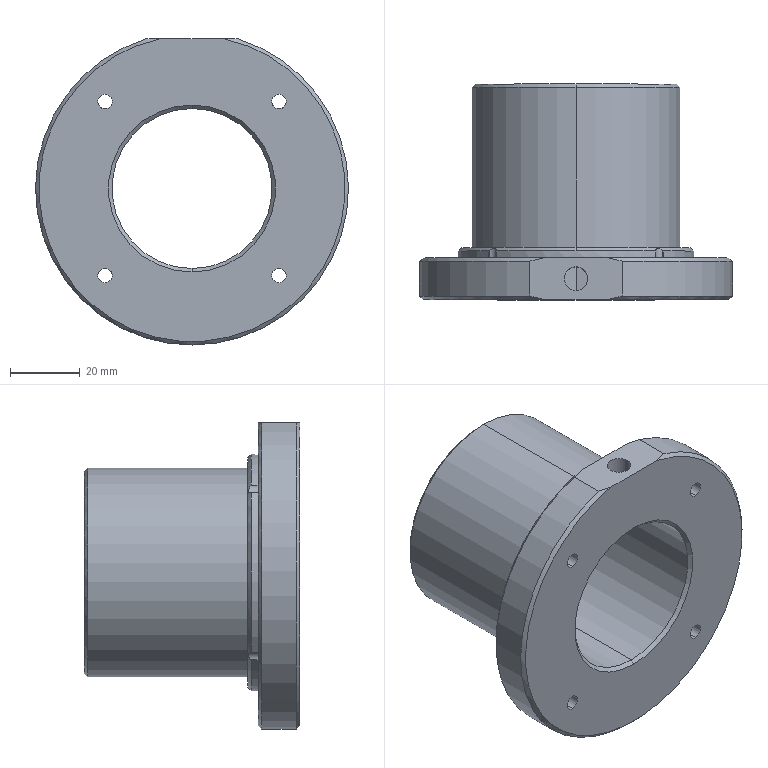Part | SolidWorks | features ICE 4, HoleWzd 2, Chamfer 1, Extrusion 1 | 1 solid | 37 faces | box 90 x 62 x 88 mm | volume 114650 mm3 | cylinder 21 | cone 11 | plane 5 | commonest cylinder face diameters 4.2 x8 68 x5 6.8 x2 46 x2 60 x2 90 x2
STEP:
#1=CARTESIAN_POINT('',(-3.4,6.,22.747));
#2=VERTEX_POINT('',#1);
#3=CARTESIAN_POINT('',(0.,2.6,23.));
#4=VERTEX_POINT('',#3);
#5=CARTESIAN_POINT('',(-3.4,6.,22.747));
#6=CARTESIAN_POINT('',(-3.4,5.778,22.747));
#7=CARTESIAN_POINT('',(-3.378,5.557,22.751));
#8=CARTESIAN_POINT('',(-3.291,5.117,22.763));
#9=CARTESIAN_POINT('',(-3.226,4.903,22.773));
#10=CARTESIAN_POINT('',(-3.056,4.494,22.796));
#11=CARTESIAN_POINT('',(-2.95,4.296,22.81));
#12=CARTESIAN_POINT('',(-2.702,3.924,22.841));
#13=CARTESIAN_POINT('',(-2.562,3.753,22.857));
#14=CARTESIAN_POINT('',(-2.248,3.44,22.89));
#15=CARTESIAN_POINT('',(-2.073,3.296,22.907));
#16=CARTESIAN_POINT('',(-1.704,3.05,22.938));
#17=CARTESIAN_POINT('',(-1.509,2.945,22.951));
#18=CARTESIAN_POINT('',(-1.097,2.774,22.975));
#19=CARTESIAN_POINT('',(-0.8814,2.709,22.984));
#20=CARTESIAN_POINT('',(-0.4465,2.622,22.997));
#21=CARTESIAN_POINT('',(-0.2248,2.6,23.));
#22=CARTESIAN_POINT('',(0.,2.6,23.));
#23=B_SPLINE_CURVE_WITH_KNOTS('',3,(#5,#6,#7,#8,#9,#10,#11,#12,#13,#14,#15,#16,#17,#18,#19,#20,#21,#22),.UNSPECIFIED.,.F.,.F.,(4,2,2,2,2,2,2,2,4),(0.01064,0.01131,0.01198,0.01264,0.01331,0.01397,0.01464,0.0153,0.01597),.UNSPECIFIED.);
#24=EDGE_CURVE('',#2,#4,#23,.T.);
#25=ORIENTED_EDGE('',*,*,#24,.F.);
#26=CARTESIAN_POINT('',(-3.4,6.,43.));
#27=VERTEX_POINT('',#26);
#28=CARTESIAN_POINT('',(-3.4,6.,43.));
#29=DIRECTION('',(0.,0.,1.));
#30=VECTOR('',#29,1000.);
#31=LINE('',#28,#30);
#32=EDGE_CURVE('',#2,#27,#31,.T.);
#33=ORIENTED_EDGE('',*,*,#32,.T.);
#34=CARTESIAN_POINT('',(3.4,6.,43.));
#35=VERTEX_POINT('',#34);
#36=CARTESIAN_POINT('',(0.,6.,43.));
#37=DIRECTION('',(0.,0.,1.));
#38=DIRECTION('',(1.,0.,0.));
#39=AXIS2_PLACEMENT_3D('',#36,#37,#38);
#40=CIRCLE('',#39,3.4);
#41=EDGE_CURVE('',#27,#35,#40,.T.);
#42=ORIENTED_EDGE('',*,*,#41,.T.);
#43=CARTESIAN_POINT('',(3.4,6.,22.747));
#44=VERTEX_POINT('',#43);
#45=CARTESIAN_POINT('',(3.4,6.,43.));
#46=DIRECTION('',(0.,0.,1.));
#47=VECTOR('',#46,1000.);
#48=LINE('',#45,#47);
#49=EDGE_CURVE('',#44,#35,#48,.T.);
#50=ORIENTED_EDGE('',*,*,#49,.F.);
#51=CARTESIAN_POINT('',(0.,2.6,23.));
#52=CARTESIAN_POINT('',(0.2246,2.6,23.));
#53=CARTESIAN_POINT('',(0.4455,2.622,22.997));
#54=CARTESIAN_POINT('',(0.8804,2.708,22.984));
#55=CARTESIAN_POINT('',(1.097,2.774,22.975));
#56=CARTESIAN_POINT('',(1.508,2.944,22.951));
#57=CARTESIAN_POINT('',(1.703,3.049,22.938));
#58=CARTESIAN_POINT('',(2.072,3.295,22.907));
#59=CARTESIAN_POINT('',(2.247,3.439,22.891));
#60=CARTESIAN_POINT('',(2.56,3.751,22.858));
#61=CARTESIAN_POINT('',(2.701,3.922,22.841));
#62=CARTESIAN_POINT('',(2.949,4.294,22.81));
#63=CARTESIAN_POINT('',(3.055,4.491,22.796));
#64=CARTESIAN_POINT('',(3.225,4.899,22.773));
#65=CARTESIAN_POINT('',(3.29,5.114,22.764));
#66=CARTESIAN_POINT('',(3.378,5.553,22.751));
#67=CARTESIAN_POINT('',(3.4,5.775,22.747));
#68=CARTESIAN_POINT('',(3.4,6.,22.747));
#69=B_SPLINE_CURVE_WITH_KNOTS('',3,(#51,#52,#53,#54,#55,#56,#57,#58,#59,#60,#61,#62,#63,#64,#65,#66,#67,#68),.UNSPECIFIED.,.F.,.F.,(4,2,2,2,2,2,2,2,4),(0.01597,0.01663,0.0173,0.01796,0.01863,0.01929,0.01996,0.02062,0.02129),.UNSPECIFIED.);
#70=EDGE_CURVE('',#4,#44,#69,.T.);
#71=ORIENTED_EDGE('',*,*,#70,.F.);
#72=EDGE_LOOP('',(#25,#33,#42,#50,#71));
#73=FACE_OUTER_BOUND('',#72,.T.);
#74=CARTESIAN_POINT('',(0.,6.,43.));
#75=DIRECTION('',(0.,0.,1.));
#76=DIRECTION('',(1.,0.,0.));
#77=AXIS2_PLACEMENT_3D('',#74,#75,#76);
#78=CYLINDRICAL_SURFACE('',#77,3.4);
#79=ADVANCED_FACE('',(#73),#78,.F.);
#80=CARTESIAN_POINT('',(-25.128,12.,22.904));
#81=VERTEX_POINT('',#80);
#82=CARTESIAN_POINT('',(-25.,12.,27.1));
#83=VERTEX_POINT('',#82);
#84=CARTESIAN_POINT('',(-25.,12.,25.));
#85=DIRECTION('',(0.,1.,0.));
#86=DIRECTION('',(0.,0.,1.));
#87=AXIS2_PLACEMENT_3D('',#84,#85,#86);
#88=CIRCLE('',#87,2.1);
#89=EDGE_CURVE('',#81,#83,#88,.T.);
#90=ORIENTED_EDGE('',*,*,#89,.T.);
#91=CARTESIAN_POINT('',(-25.,0.,27.1));
#92=VERTEX_POINT('',#91);
#93=CARTESIAN_POINT('',(-25.,0.,27.1));
#94=DIRECTION('',(0.,-1.,0.));
#95=VECTOR('',#94,1000.);
#96=LINE('',#93,#95);
#97=EDGE_CURVE('',#83,#92,#96,.T.);
#98=ORIENTED_EDGE('',*,*,#97,.T.);
#99=CARTESIAN_POINT('',(-25.,0.,22.9));
#100=VERTEX_POINT('',#99);
#101=CARTESIAN_POINT('',(-25.,0.,25.));
#102=DIRECTION('',(0.,-1.,0.));
#103=DIRECTION('',(0.,0.,-1.));
#104=AXIS2_PLACEMENT_3D('',#101,#102,#103);
#105=CIRCLE('',#104,2.1);
#106=EDGE_CURVE('',#92,#100,#105,.T.);
#107=ORIENTED_EDGE('',*,*,#106,.T.);
#108=CARTESIAN_POINT('',(-25.,14.097,22.9));
#109=VERTEX_POINT('',#108);
#110=CARTESIAN_POINT('',(-25.,0.,22.9));
#111=DIRECTION('',(0.,-1.,0.));
#112=VECTOR('',#111,1000.);
#113=LINE('',#110,#112);
#114=EDGE_CURVE('',#109,#100,#113,.T.);
#115=ORIENTED_EDGE('',*,*,#114,.F.);
#116=CARTESIAN_POINT('',(-25.128,14.,22.904));
#117=VERTEX_POINT('',#116);
#118=CARTESIAN_POINT('',(-25.,14.097,22.9));
#119=CARTESIAN_POINT('',(-25.043,14.065,22.9));
#120=CARTESIAN_POINT('',(-25.086,14.033,22.901));
#121=CARTESIAN_POINT('',(-25.128,14.,22.904));
#122=B_SPLINE_CURVE_WITH_KNOTS('',3,(#118,#119,#120,#121),.UNSPECIFIED.,.F.,.F.,(4,4),(0.003743,0.003902),.UNSPECIFIED.);
#123=EDGE_CURVE('',#109,#117,#122,.T.);
#124=ORIENTED_EDGE('',*,*,#123,.T.);
#125=CARTESIAN_POINT('',(-25.128,31.,22.904));
#126=DIRECTION('',(0.,1.,0.));
#127=VECTOR('',#126,1000.);
#128=LINE('',#125,#127);
#129=EDGE_CURVE('',#81,#117,#128,.T.);
#130=ORIENTED_EDGE('',*,*,#129,.F.);
#131=EDGE_LOOP('',(#90,#98,#107,#115,#124,#130));
#132=FACE_OUTER_BOUND('',#131,.T.);
#133=CARTESIAN_POINT('',(-25.,0.,25.));
#134=DIRECTION('',(0.,-1.,0.));
#135=DIRECTION('',(0.,0.,-1.));
#136=AXIS2_PLACEMENT_3D('',#133,#134,#135);
#137=CYLINDRICAL_SURFACE('',#136,2.1);
#138=ADVANCED_FACE('',(#132),#137,.F.);
#139=CARTESIAN_POINT('',(22.904,12.,25.128));
#140=VERTEX_POINT('',#139);
#141=CARTESIAN_POINT('',(25.,12.,27.1));
#142=VERTEX_POINT('',#141);
#143=CARTESIAN_POINT('',(25.,12.,25.));
#144=DIRECTION('',(0.,1.,0.));
#145=DIRECTION('',(0.,0.,1.));
#146=AXIS2_PLACEMENT_3D('',#143,#144,#145);
#147=CIRCLE('',#146,2.1);
#148=EDGE_CURVE('',#140,#142,#147,.T.);
#149=ORIENTED_EDGE('',*,*,#148,.T.);
#150=CARTESIAN_POINT('',(25.,0.,27.1));
#151=VERTEX_POINT('',#150);
#152=CARTESIAN_POINT('',(25.,0.,27.1));
#153=DIRECTION('',(0.,-1.,0.));
#154=VECTOR('',#153,1000.);
#155=LINE('',#152,#154);
#156=EDGE_CURVE('',#142,#151,#155,.T.);
#157=ORIENTED_EDGE('',*,*,#156,.T.);
#158=CARTESIAN_POINT('',(25.,0.,22.9));
#159=VERTEX_POINT('',#158);
#160=CARTESIAN_POINT('',(25.,0.,25.));
#161=DIRECTION('',(0.,-1.,0.));
#162=DIRECTION('',(0.,0.,-1.));
#163=AXIS2_PLACEMENT_3D('',#160,#161,#162);
#164=CIRCLE('',#163,2.1);
#165=EDGE_CURVE('',#151,#159,#164,.T.);
#166=ORIENTED_EDGE('',*,*,#165,.T.);
#167=CARTESIAN_POINT('',(25.,14.097,22.9));
#168=VERTEX_POINT('',#167);
#169=CARTESIAN_POINT('',(25.,0.,22.9));
#170=DIRECTION('',(0.,-1.,0.));
#171=VECTOR('',#170,1000.);
#172=LINE('',#169,#171);
#173=EDGE_CURVE('',#168,#159,#172,.T.);
#174=ORIENTED_EDGE('',*,*,#173,.F.);
#175=CARTESIAN_POINT('',(22.904,14.,25.128));
#176=VERTEX_POINT('',#175);
#177=CARTESIAN_POINT('',(25.,14.097,22.9));
#178=CARTESIAN_POINT('',(24.874,14.19,22.9));
#179=CARTESIAN_POINT('',(24.745,14.277,22.911));
#180=CARTESIAN_POINT('',(24.48,14.437,22.961));
#181=CARTESIAN_POINT('',(24.344,14.51,23.));
#182=CARTESIAN_POINT('',(24.076,14.628,23.108));
#183=CARTESIAN_POINT('',(23.941,14.676,23.18));
#184=CARTESIAN_POINT('',(23.688,14.736,23.353));
#185=CARTESIAN_POINT('',(23.567,14.749,23.457));
#186=CARTESIAN_POINT('',(23.354,14.737,23.687));
#187=CARTESIAN_POINT('',(23.261,14.712,23.814));
#188=CARTESIAN_POINT('',(23.108,14.629,24.076));
#189=CARTESIAN_POINT('',(23.048,14.572,24.212));
#190=CARTESIAN_POINT('',(22.916,14.369,24.616));
#191=CARTESIAN_POINT('',(22.889,14.194,24.879));
#192=CARTESIAN_POINT('',(22.904,14.,25.128));
#193=B_SPLINE_CURVE_WITH_KNOTS('',3,(#177,#178,#179,#180,#181,#182,#183,#184,#185,#186,#187,#188,#189,#190,#191,#192),.UNSPECIFIED.,.F.,.F.,(4,2,2,2,2,2,2,4),(0.0001598,0.0006275,0.001095,0.001563,0.002031,0.002499,0.002966,0.003902),.UNSPECIFIED.);
#194=EDGE_CURVE('',#168,#176,#193,.T.);
#195=ORIENTED_EDGE('',*,*,#194,.T.);
#196=CARTESIAN_POINT('',(22.904,31.,25.128));
#197=DIRECTION('',(0.,1.,0.));
#198=VECTOR('',#197,1000.);
#199=LINE('',#196,#198);
#200=EDGE_CURVE('',#140,#176,#199,.T.);
#201=ORIENTED_EDGE('',*,*,#200,.F.);
#202=EDGE_LOOP('',(#149,#157,#166,#174,#195,#201));
#203=FACE_OUTER_BOUND('',#202,.T.);
#204=CARTESIAN_POINT('',(25.,0.,25.));
#205=DIRECTION('',(0.,-1.,0.));
#206=DIRECTION('',(0.,0.,-1.));
#207=AXIS2_PLACEMENT_3D('',#204,#205,#206);
#208=CYLINDRICAL_SURFACE('',#207,2.1);
#209=ADVANCED_FACE('',(#203),#208,.F.);
#210=CARTESIAN_POINT('',(22.904,14.,-25.128));
#211=VERTEX_POINT('',#210);
#212=CARTESIAN_POINT('',(25.,14.097,-22.9));
#213=VERTEX_POINT('',#212);
#214=CARTESIAN_POINT('',(22.904,14.,-25.128));
#215=CARTESIAN_POINT('',(22.896,14.097,-25.004));
#216=CARTESIAN_POINT('',(22.9,14.188,-24.877));
#217=CARTESIAN_POINT('',(22.931,14.358,-24.617));
#218=CARTESIAN_POINT('',(22.96,14.437,-24.482));
#219=CARTESIAN_POINT('',(23.092,14.639,-24.078));
#220=CARTESIAN_POINT('',(23.243,14.73,-23.806));
#221=CARTESIAN_POINT('',(23.674,14.756,-23.341));
#222=CARTESIAN_POINT('',(23.938,14.69,-23.165));
#223=CARTESIAN_POINT('',(24.479,14.45,-22.945));
#224=CARTESIAN_POINT('',(24.746,14.284,-22.9));
#225=CARTESIAN_POINT('',(25.,14.097,-22.9));
#226=B_SPLINE_CURVE_WITH_KNOTS('',3,(#214,#215,#216,#217,#218,#219,#220,#221,#222,#223,#224,#225),.UNSPECIFIED.,.F.,.F.,(4,2,2,2,2,4),(0.000000322,0.0004682,0.000936,0.001872,0.002807,0.003743),.UNSPECIFIED.);
#227=EDGE_CURVE('',#211,#213,#226,.T.);
#228=ORIENTED_EDGE('',*,*,#227,.T.);
#229=CARTESIAN_POINT('',(25.,0.,-22.9));
#230=VERTEX_POINT('',#229);
#231=CARTESIAN_POINT('',(25.,0.,-22.9));
#232=DIRECTION('',(0.,-1.,0.));
#233=VECTOR('',#232,1000.);
#234=LINE('',#231,#233);
#235=EDGE_CURVE('',#213,#230,#234,.T.);
#236=ORIENTED_EDGE('',*,*,#235,.T.);
#237=CARTESIAN_POINT('',(25.,0.,-27.1));
#238=VERTEX_POINT('',#237);
#239=CARTESIAN_POINT('',(25.,0.,-25.));
#240=DIRECTION('',(0.,-1.,0.));
#241=DIRECTION('',(0.,0.,-1.));
#242=AXIS2_PLACEMENT_3D('',#239,#240,#241);
#243=CIRCLE('',#242,2.1);
#244=EDGE_CURVE('',#230,#238,#243,.T.);
#245=ORIENTED_EDGE('',*,*,#244,.T.);
#246=CARTESIAN_POINT('',(25.,12.,-27.1));
#247=VERTEX_POINT('',#246);
#248=CARTESIAN_POINT('',(25.,0.,-27.1));
#249=DIRECTION('',(0.,-1.,0.));
#250=VECTOR('',#249,1000.);
#251=LINE('',#248,#250);
#252=EDGE_CURVE('',#247,#238,#251,.T.);
#253=ORIENTED_EDGE('',*,*,#252,.F.);
#254=CARTESIAN_POINT('',(22.904,12.,-25.128));
#255=VERTEX_POINT('',#254);
#256=CARTESIAN_POINT('',(25.,12.,-25.));
#257=DIRECTION('',(0.,1.,0.));
#258=DIRECTION('',(0.,0.,1.));
#259=AXIS2_PLACEMENT_3D('',#256,#257,#258);
#260=CIRCLE('',#259,2.1);
#261=EDGE_CURVE('',#247,#255,#260,.T.);
#262=ORIENTED_EDGE('',*,*,#261,.T.);
#263=CARTESIAN_POINT('',(22.904,31.,-25.128));
#264=DIRECTION('',(0.,-1.,0.));
#265=VECTOR('',#264,1000.);
#266=LINE('',#263,#265);
#267=EDGE_CURVE('',#211,#255,#266,.T.);
#268=ORIENTED_EDGE('',*,*,#267,.F.);
#269=EDGE_LOOP('',(#228,#236,#245,#253,#262,#268));
#270=FACE_OUTER_BOUND('',#269,.T.);
#271=CARTESIAN_POINT('',(25.,0.,-25.));
#272=DIRECTION('',(0.,-1.,0.));
#273=DIRECTION('',(0.,0.,-1.));
#274=AXIS2_PLACEMENT_3D('',#271,#272,#273);
#275=CYLINDRICAL_SURFACE('',#274,2.1);
#276=ADVANCED_FACE('',(#270),#275,.F.);
#277=CARTESIAN_POINT('',(-25.128,14.,-22.904));
#278=VERTEX_POINT('',#277);
#279=CARTESIAN_POINT('',(-25.,14.097,-22.9));
#280=VERTEX_POINT('',#279);
#281=CARTESIAN_POINT('',(-25.128,14.,-22.904));
#282=CARTESIAN_POINT('',(-25.086,14.033,-22.901));
#283=CARTESIAN_POINT('',(-25.043,14.065,-22.9));
#284=CARTESIAN_POINT('',(-25.,14.097,-22.9));
#285=B_SPLINE_CURVE_WITH_KNOTS('',3,(#281,#282,#283,#284),.UNSPECIFIED.,.F.,.F.,(4,4),(0.000000322,0.0001598),.UNSPECIFIED.);
#286=EDGE_CURVE('',#278,#280,#285,.T.);
#287=ORIENTED_EDGE('',*,*,#286,.T.);
#288=CARTESIAN_POINT('',(-25.,0.,-22.9));
#289=VERTEX_POINT('',#288);
#290=CARTESIAN_POINT('',(-25.,0.,-22.9));
#291=DIRECTION('',(0.,-1.,0.));
#292=VECTOR('',#291,1000.);
#293=LINE('',#290,#292);
#294=EDGE_CURVE('',#280,#289,#293,.T.);
#295=ORIENTED_EDGE('',*,*,#294,.T.);
#296=CARTESIAN_POINT('',(-25.,0.,-27.1));
#297=VERTEX_POINT('',#296);
#298=CARTESIAN_POINT('',(-25.,0.,-25.));
#299=DIRECTION('',(0.,-1.,0.));
#300=DIRECTION('',(0.,0.,-1.));
#301=AXIS2_PLACEMENT_3D('',#298,#299,#300);
#302=CIRCLE('',#301,2.1);
#303=EDGE_CURVE('',#289,#297,#302,.T.);
#304=ORIENTED_EDGE('',*,*,#303,.T.);
#305=CARTESIAN_POINT('',(-25.,12.,-27.1));
#306=VERTEX_POINT('',#305);
#307=CARTESIAN_POINT('',(-25.,0.,-27.1));
#308=DIRECTION('',(0.,-1.,0.));
#309=VECTOR('',#308,1000.);
#310=LINE('',#307,#309);
#311=EDGE_CURVE('',#306,#297,#310,.T.);
#312=ORIENTED_EDGE('',*,*,#311,.F.);
#313=CARTESIAN_POINT('',(-25.128,12.,-22.904));
#314=VERTEX_POINT('',#313);
#315=CARTESIAN_POINT('',(-25.,12.,-25.));
#316=DIRECTION('',(0.,1.,0.));
#317=DIRECTION('',(0.,0.,1.));
#318=AXIS2_PLACEMENT_3D('',#315,#316,#317);
#319=CIRCLE('',#318,2.1);
#320=EDGE_CURVE('',#306,#314,#319,.T.);
#321=ORIENTED_EDGE('',*,*,#320,.T.);
#322=CARTESIAN_POINT('',(-25.128,31.,-22.904));
#323=DIRECTION('',(0.,-1.,0.));
#324=VECTOR('',#323,1000.);
#325=LINE('',#322,#324);
#326=EDGE_CURVE('',#278,#314,#325,.T.);
#327=ORIENTED_EDGE('',*,*,#326,.F.);
#328=EDGE_LOOP('',(#287,#295,#304,#312,#321,#327));
#329=FACE_OUTER_BOUND('',#328,.T.);
#330=CARTESIAN_POINT('',(-25.,0.,-25.));
#331=DIRECTION('',(0.,-1.,0.));
#332=DIRECTION('',(0.,0.,-1.));
#333=AXIS2_PLACEMENT_3D('',#330,#331,#332);
#334=CYLINDRICAL_SURFACE('',#333,2.1);
#335=ADVANCED_FACE('',(#329),#334,.F.);
#336=CARTESIAN_POINT('',(0.,62.,29.));
#337=VERTEX_POINT('',#336);
#338=CARTESIAN_POINT('',(0.,62.,-29.));
#339=VERTEX_POINT('',#338);
#340=CARTESIAN_POINT('',(0.,62.,0.));
#341=DIRECTION('',(0.,1.,0.));
#342=DIRECTION('',(0.,0.,1.));
#343=AXIS2_PLACEMENT_3D('',#340,#341,#342);
#344=CIRCLE('',#343,29.);
#345=EDGE_CURVE('',#337,#339,#344,.T.);
#346=ORIENTED_EDGE('',*,*,#345,.F.);
#347=CARTESIAN_POINT('',(0.,61.,30.));
#348=VERTEX_POINT('',#347);
#349=CARTESIAN_POINT('',(0.,62.,29.));
#350=DIRECTION('',(0.,-0.7071,0.7071));
#351=VECTOR('',#350,1000.);
#352=LINE('',#349,#351);
#353=EDGE_CURVE('',#337,#348,#352,.T.);
#354=ORIENTED_EDGE('',*,*,#353,.T.);
#355=CARTESIAN_POINT('',(0.,61.,-30.));
#356=VERTEX_POINT('',#355);
#357=CARTESIAN_POINT('',(0.,61.,0.));
#358=DIRECTION('',(0.,-1.,0.));
#359=DIRECTION('',(0.,0.,1.));
#360=AXIS2_PLACEMENT_3D('',#357,#358,#359);
#361=CIRCLE('',#360,30.);
#362=EDGE_CURVE('',#356,#348,#361,.T.);
#363=ORIENTED_EDGE('',*,*,#362,.F.);
#364=CARTESIAN_POINT('',(0.,62.,-29.));
#365=DIRECTION('',(0.,-0.7071,-0.7071));
#366=VECTOR('',#365,1000.);
#367=LINE('',#364,#366);
#368=EDGE_CURVE('',#339,#356,#367,.T.);
#369=ORIENTED_EDGE('',*,*,#368,.F.);
#370=EDGE_LOOP('',(#346,#354,#363,#369));
#371=FACE_OUTER_BOUND('',#370,.T.);
#372=CARTESIAN_POINT('',(0.,62.,0.));
#373=DIRECTION('',(0.,-1.,0.));
#374=DIRECTION('',(0.,0.,-1.));
#375=AXIS2_PLACEMENT_3D('',#372,#373,#374);
#376=CONICAL_SURFACE('',#375,29.,0.7854);
#377=ADVANCED_FACE('',(#371),#376,.T.);
#378=CARTESIAN_POINT('',(0.,12.,-44.));
#379=VERTEX_POINT('',#378);
#380=CARTESIAN_POINT('',(-9.327,12.,43.));
#381=VERTEX_POINT('',#380);
#382=CARTESIAN_POINT('',(0.,12.,0.));
#383=DIRECTION('',(0.,1.,0.));
#384=DIRECTION('',(0.,0.,1.));
#385=AXIS2_PLACEMENT_3D('',#382,#383,#384);
#386=CIRCLE('',#385,44.);
#387=EDGE_CURVE('',#379,#381,#386,.T.);
#388=ORIENTED_EDGE('',*,*,#387,.F.);
#389=CARTESIAN_POINT('',(0.,11.,-45.));
#390=VERTEX_POINT('',#389);
#391=CARTESIAN_POINT('',(0.,12.,-44.));
#392=DIRECTION('',(0.,-0.7071,-0.7071));
#393=VECTOR('',#392,1000.);
#394=LINE('',#391,#393);
#395=EDGE_CURVE('',#379,#390,#394,.T.);
#396=ORIENTED_EDGE('',*,*,#395,.T.);
#397=CARTESIAN_POINT('',(-13.266,11.,43.));
#398=VERTEX_POINT('',#397);
#399=CARTESIAN_POINT('',(0.,11.,0.));
#400=DIRECTION('',(0.,-1.,0.));
#401=DIRECTION('',(0.,0.,1.));
#402=AXIS2_PLACEMENT_3D('',#399,#400,#401);
#403=CIRCLE('',#402,45.);
#404=EDGE_CURVE('',#398,#390,#403,.T.);
#405=ORIENTED_EDGE('',*,*,#404,.F.);
#406=CARTESIAN_POINT('',(-9.327,12.,43.));
#407=CARTESIAN_POINT('',(-10.657,11.718,43.));
#408=CARTESIAN_POINT('',(-11.969,11.382,43.));
#409=CARTESIAN_POINT('',(-13.266,11.,43.));
#410=B_SPLINE_CURVE_WITH_KNOTS('',3,(#406,#407,#408,#409),.UNSPECIFIED.,.F.,.F.,(4,4),(0.04009,0.04415),.UNSPECIFIED.);
#411=EDGE_CURVE('',#381,#398,#410,.T.);
#412=ORIENTED_EDGE('',*,*,#411,.F.);
#413=EDGE_LOOP('',(#388,#396,#405,#412));
#414=FACE_OUTER_BOUND('',#413,.T.);
#415=CARTESIAN_POINT('',(0.,12.,0.));
#416=DIRECTION('',(0.,-1.,0.));
#417=DIRECTION('',(0.,0.,-1.));
#418=AXIS2_PLACEMENT_3D('',#415,#416,#417);
#419=CONICAL_SURFACE('',#418,44.,0.7854);
#420=ADVANCED_FACE('',(#414),#419,.T.);
#421=CARTESIAN_POINT('',(0.,1.,23.));
#422=VERTEX_POINT('',#421);
#423=CARTESIAN_POINT('',(0.,1.,-23.));
#424=VERTEX_POINT('',#423);
#425=CARTESIAN_POINT('',(0.,1.,0.));
#426=DIRECTION('',(0.,-1.,0.));
#427=DIRECTION('',(0.,0.,1.));
#428=AXIS2_PLACEMENT_3D('',#425,#426,#427);
#429=CIRCLE('',#428,23.);
#430=EDGE_CURVE('',#422,#424,#429,.T.);
#431=ORIENTED_EDGE('',*,*,#430,.F.);
#432=CARTESIAN_POINT('',(0.,0.,24.));
#433=VERTEX_POINT('',#432);
#434=CARTESIAN_POINT('',(0.,1.,23.));
#435=DIRECTION('',(0.,-0.7071,0.7071));
#436=VECTOR('',#435,1000.);
#437=LINE('',#434,#436);
#438=EDGE_CURVE('',#422,#433,#437,.T.);
#439=ORIENTED_EDGE('',*,*,#438,.T.);
#440=CARTESIAN_POINT('',(0.,0.,-24.));
#441=VERTEX_POINT('',#440);
#442=CARTESIAN_POINT('',(0.,0.,0.));
#443=DIRECTION('',(0.,1.,0.));
#444=DIRECTION('',(0.,0.,1.));
#445=AXIS2_PLACEMENT_3D('',#442,#443,#444);
#446=CIRCLE('',#445,24.);
#447=EDGE_CURVE('',#441,#433,#446,.T.);
#448=ORIENTED_EDGE('',*,*,#447,.F.);
#449=CARTESIAN_POINT('',(0.,1.,-23.));
#450=DIRECTION('',(0.,-0.7071,-0.7071));
#451=VECTOR('',#450,1000.);
#452=LINE('',#449,#451);
#453=EDGE_CURVE('',#424,#441,#452,.T.);
#454=ORIENTED_EDGE('',*,*,#453,.F.);
#455=EDGE_LOOP('',(#431,#439,#448,#454));
#456=FACE_OUTER_BOUND('',#455,.T.);
#457=CARTESIAN_POINT('',(0.,1.,0.));
#458=DIRECTION('',(0.,-1.,0.));
#459=DIRECTION('',(0.,0.,-1.));
#460=AXIS2_PLACEMENT_3D('',#457,#458,#459);
#461=CONICAL_SURFACE('',#460,23.,0.7854);
#462=ADVANCED_FACE('',(#456),#461,.F.);
#463=CARTESIAN_POINT('',(0.,61.,-23.));
#464=VERTEX_POINT('',#463);
#465=CARTESIAN_POINT('',(0.,61.,23.));
#466=VERTEX_POINT('',#465);
#467=CARTESIAN_POINT('',(0.,61.,0.));
#468=DIRECTION('',(0.,1.,0.));
#469=DIRECTION('',(0.,0.,1.));
#470=AXIS2_PLACEMENT_3D('',#467,#468,#469);
#471=CIRCLE('',#470,23.);
#472=EDGE_CURVE('',#464,#466,#471,.T.);
#473=ORIENTED_EDGE('',*,*,#472,.F.);
#474=CARTESIAN_POINT('',(0.,62.,-24.));
#475=VERTEX_POINT('',#474);
#476=CARTESIAN_POINT('',(0.,62.,-24.));
#477=DIRECTION('',(0.,0.7071,-0.7071));
#478=VECTOR('',#477,1000.);
#479=LINE('',#476,#478);
#480=EDGE_CURVE('',#464,#475,#479,.T.);
#481=ORIENTED_EDGE('',*,*,#480,.T.);
#482=CARTESIAN_POINT('',(0.,62.,24.));
#483=VERTEX_POINT('',#482);
#484=CARTESIAN_POINT('',(0.,62.,0.));
#485=DIRECTION('',(0.,-1.,0.));
#486=DIRECTION('',(0.,0.,1.));
#487=AXIS2_PLACEMENT_3D('',#484,#485,#486);
#488=CIRCLE('',#487,24.);
#489=EDGE_CURVE('',#483,#475,#488,.T.);
#490=ORIENTED_EDGE('',*,*,#489,.F.);
#491=CARTESIAN_POINT('',(0.,62.,24.));
#492=DIRECTION('',(0.,0.7071,0.7071));
#493=VECTOR('',#492,1000.);
#494=LINE('',#491,#493);
#495=EDGE_CURVE('',#466,#483,#494,.T.);
#496=ORIENTED_EDGE('',*,*,#495,.F.);
#497=EDGE_LOOP('',(#473,#481,#490,#496));
#498=FACE_OUTER_BOUND('',#497,.T.);
#499=CARTESIAN_POINT('',(0.,62.,0.));
#500=DIRECTION('',(0.,1.,0.));
#501=DIRECTION('',(0.,0.,1.));
#502=AXIS2_PLACEMENT_3D('',#499,#500,#501);
#503=CONICAL_SURFACE('',#502,24.,0.7854);
#504=ADVANCED_FACE('',(#498),#503,.F.);
#505=CARTESIAN_POINT('',(0.,15.,33.));
#506=VERTEX_POINT('',#505);
#507=CARTESIAN_POINT('',(0.,15.,-33.));
#508=VERTEX_POINT('',#507);
#509=CARTESIAN_POINT('',(0.,15.,0.));
#510=DIRECTION('',(0.,1.,0.));
#511=DIRECTION('',(0.,0.,1.));
#512=AXIS2_PLACEMENT_3D('',#509,#510,#511);
#513=CIRCLE('',#512,33.);
#514=EDGE_CURVE('',#506,#508,#513,.T.);
#515=ORIENTED_EDGE('',*,*,#514,.F.);
#516=CARTESIAN_POINT('',(0.,14.,34.));
#517=VERTEX_POINT('',#516);
#518=CARTESIAN_POINT('',(0.,15.,33.));
#519=DIRECTION('',(0.,-0.7071,0.7071));
#520=VECTOR('',#519,1000.);
#521=LINE('',#518,#520);
#522=EDGE_CURVE('',#506,#517,#521,.T.);
#523=ORIENTED_EDGE('',*,*,#522,.T.);
#524=CARTESIAN_POINT('',(0.,14.,0.));
#525=DIRECTION('',(0.,-1.,0.));
#526=DIRECTION('',(0.,0.,1.));
#527=AXIS2_PLACEMENT_3D('',#524,#525,#526);
#528=CIRCLE('',#527,34.);
#529=EDGE_CURVE('',#176,#517,#528,.T.);
#530=ORIENTED_EDGE('',*,*,#529,.F.);
#531=ORIENTED_EDGE('',*,*,#194,.F.);
#532=CARTESIAN_POINT('',(25.128,14.,22.904));
#533=VERTEX_POINT('',#532);
#534=CARTESIAN_POINT('',(25.128,14.,22.904));
#535=CARTESIAN_POINT('',(25.086,14.033,22.901));
#536=CARTESIAN_POINT('',(25.043,14.065,22.9));
#537=CARTESIAN_POINT('',(25.,14.097,22.9));
#538=B_SPLINE_CURVE_WITH_KNOTS('',3,(#534,#535,#536,#537),.UNSPECIFIED.,.F.,.F.,(4,4),(0.000000322,0.0001598),.UNSPECIFIED.);
#539=EDGE_CURVE('',#533,#168,#538,.T.);
#540=ORIENTED_EDGE('',*,*,#539,.F.);
#541=CARTESIAN_POINT('',(25.128,14.,-22.904));
#542=VERTEX_POINT('',#541);
#543=CARTESIAN_POINT('',(0.,14.,0.));
#544=DIRECTION('',(0.,-1.,0.));
#545=DIRECTION('',(0.,0.,1.));
#546=AXIS2_PLACEMENT_3D('',#543,#544,#545);
#547=CIRCLE('',#546,34.);
#548=EDGE_CURVE('',#542,#533,#547,.T.);
#549=ORIENTED_EDGE('',*,*,#548,.F.);
#550=CARTESIAN_POINT('',(25.,14.097,-22.9));
#551=CARTESIAN_POINT('',(25.043,14.065,-22.9));
#552=CARTESIAN_POINT('',(25.086,14.033,-22.901));
#553=CARTESIAN_POINT('',(25.128,14.,-22.904));
#554=B_SPLINE_CURVE_WITH_KNOTS('',3,(#550,#551,#552,#553),.UNSPECIFIED.,.F.,.F.,(4,4),(0.003743,0.003902),.UNSPECIFIED.);
#555=EDGE_CURVE('',#213,#542,#554,.T.);
#556=ORIENTED_EDGE('',*,*,#555,.F.);
#557=ORIENTED_EDGE('',*,*,#227,.F.);
#558=CARTESIAN_POINT('',(0.,14.,-34.));
#559=VERTEX_POINT('',#558);
#560=CARTESIAN_POINT('',(0.,14.,0.));
#561=DIRECTION('',(0.,-1.,0.));
#562=DIRECTION('',(0.,0.,1.));
#563=AXIS2_PLACEMENT_3D('',#560,#561,#562);
#564=CIRCLE('',#563,34.);
#565=EDGE_CURVE('',#559,#211,#564,.T.);
#566=ORIENTED_EDGE('',*,*,#565,.F.);
#567=CARTESIAN_POINT('',(0.,15.,-33.));
#568=DIRECTION('',(0.,-0.7071,-0.7071));
#569=VECTOR('',#568,1000.);
#570=LINE('',#567,#569);
#571=EDGE_CURVE('',#508,#559,#570,.T.);
#572=ORIENTED_EDGE('',*,*,#571,.F.);
#573=EDGE_LOOP('',(#515,#523,#530,#531,#540,#549,#556,#557,#566,#572));
#574=FACE_OUTER_BOUND('',#573,.T.);
#575=CARTESIAN_POINT('',(0.,15.,0.));
#576=DIRECTION('',(0.,-1.,0.));
#577=DIRECTION('',(0.,0.,-1.));
#578=AXIS2_PLACEMENT_3D('',#575,#576,#577);
#579=CONICAL_SURFACE('',#578,33.,0.7854);
#580=ADVANCED_FACE('',(#574),#579,.T.);
#581=ORIENTED_EDGE('',*,*,#472,.T.);
#582=CARTESIAN_POINT('',(0.,9.4,23.));
#583=VERTEX_POINT('',#582);
#584=CARTESIAN_POINT('',(0.,62.,23.));
#585=DIRECTION('',(0.,-1.,0.));
#586=VECTOR('',#585,1000.);
#587=LINE('',#584,#586);
#588=EDGE_CURVE('',#466,#583,#587,.T.);
#589=ORIENTED_EDGE('',*,*,#588,.T.);
#590=CARTESIAN_POINT('',(0.,9.4,23.));
#591=CARTESIAN_POINT('',(-0.2221,9.4,23.));
#592=CARTESIAN_POINT('',(-0.4476,9.378,22.997));
#593=CARTESIAN_POINT('',(-0.8838,9.291,22.984));
#594=CARTESIAN_POINT('',(-1.096,9.226,22.975));
#595=CARTESIAN_POINT('',(-1.508,9.056,22.951));
#596=CARTESIAN_POINT('',(-1.706,8.949,22.937));
#597=CARTESIAN_POINT('',(-2.074,8.703,22.907));
#598=CARTESIAN_POINT('',(-2.246,8.562,22.891));
#599=CARTESIAN_POINT('',(-2.563,8.245,22.857));
#600=CARTESIAN_POINT('',(-2.703,8.074,22.841));
#601=CARTESIAN_POINT('',(-2.949,7.706,22.81));
#602=CARTESIAN_POINT('',(-3.056,7.507,22.796));
#603=CARTESIAN_POINT('',(-3.226,7.096,22.773));
#604=CARTESIAN_POINT('',(-3.291,6.884,22.763));
#605=CARTESIAN_POINT('',(-3.378,6.448,22.751));
#606=CARTESIAN_POINT('',(-3.4,6.222,22.747));
#607=CARTESIAN_POINT('',(-3.4,6.,22.747));
#608=B_SPLINE_CURVE_WITH_KNOTS('',3,(#590,#591,#592,#593,#594,#595,#596,#597,#598,#599,#600,#601,#602,#603,#604,#605,#606,#607),.UNSPECIFIED.,.F.,.F.,(4,2,2,2,2,2,2,2,4),(0.005324,0.005989,0.006654,0.007319,0.007984,0.008649,0.009314,0.009979,0.01064),.UNSPECIFIED.);
#609=EDGE_CURVE('',#583,#2,#608,.T.);
#610=ORIENTED_EDGE('',*,*,#609,.T.);
#611=ORIENTED_EDGE('',*,*,#24,.T.);
#612=CARTESIAN_POINT('',(0.,62.,23.));
#613=DIRECTION('',(0.,-1.,0.));
#614=VECTOR('',#613,1000.);
#615=LINE('',#612,#614);
#616=EDGE_CURVE('',#4,#422,#615,.T.);
#617=ORIENTED_EDGE('',*,*,#616,.T.);
#618=ORIENTED_EDGE('',*,*,#430,.T.);
#619=CARTESIAN_POINT('',(0.,62.,-23.));
#620=DIRECTION('',(0.,-1.,0.));
#621=VECTOR('',#620,1000.);
#622=LINE('',#619,#621);
#623=EDGE_CURVE('',#464,#424,#622,.T.);
#624=ORIENTED_EDGE('',*,*,#623,.F.);
#625=EDGE_LOOP('',(#581,#589,#610,#611,#617,#618,#624));
#626=FACE_OUTER_BOUND('',#625,.T.);
#627=CARTESIAN_POINT('',(0.,62.,0.));
#628=DIRECTION('',(0.,-1.,0.));
#629=DIRECTION('',(0.,0.,-1.));
#630=AXIS2_PLACEMENT_3D('',#627,#628,#629);
#631=CYLINDRICAL_SURFACE('',#630,23.);
#632=ADVANCED_FACE('',(#626),#631,.F.);
#633=ORIENTED_EDGE('',*,*,#362,.T.);
#634=CARTESIAN_POINT('',(0.,15.,30.));
#635=VERTEX_POINT('',#634);
#636=CARTESIAN_POINT('',(0.,62.,30.));
#637=DIRECTION('',(0.,-1.,0.));
#638=VECTOR('',#637,1000.);
#639=LINE('',#636,#638);
#640=EDGE_CURVE('',#348,#635,#639,.T.);
#641=ORIENTED_EDGE('',*,*,#640,.T.);
#642=CARTESIAN_POINT('',(0.,15.,-30.));
#643=VERTEX_POINT('',#642);
#644=CARTESIAN_POINT('',(0.,15.,0.));
#645=DIRECTION('',(0.,1.,0.));
#646=DIRECTION('',(0.,0.,1.));
#647=AXIS2_PLACEMENT_3D('',#644,#645,#646);
#648=CIRCLE('',#647,30.);
#649=EDGE_CURVE('',#635,#643,#648,.T.);
#650=ORIENTED_EDGE('',*,*,#649,.T.);
#651=CARTESIAN_POINT('',(0.,62.,-30.));
#652=DIRECTION('',(0.,-1.,0.));
#653=VECTOR('',#652,1000.);
#654=LINE('',#651,#653);
#655=EDGE_CURVE('',#356,#643,#654,.T.);
#656=ORIENTED_EDGE('',*,*,#655,.F.);
#657=EDGE_LOOP('',(#633,#641,#650,#656));
#658=FACE_OUTER_BOUND('',#657,.T.);
#659=CARTESIAN_POINT('',(0.,62.,0.));
#660=DIRECTION('',(0.,-1.,0.));
#661=DIRECTION('',(0.,0.,-1.));
#662=AXIS2_PLACEMENT_3D('',#659,#660,#661);
#663=CYLINDRICAL_SURFACE('',#662,30.);
#664=ADVANCED_FACE('',(#658),#663,.T.);
#665=CARTESIAN_POINT('',(-22.904,14.,-25.128));
#666=VERTEX_POINT('',#665);
#667=CARTESIAN_POINT('',(0.,14.,0.));
#668=DIRECTION('',(0.,-1.,0.));
#669=DIRECTION('',(0.,0.,1.));
#670=AXIS2_PLACEMENT_3D('',#667,#668,#669);
#671=CIRCLE('',#670,34.);
#672=EDGE_CURVE('',#666,#559,#671,.T.);
#673=ORIENTED_EDGE('',*,*,#672,.T.);
#674=CARTESIAN_POINT('',(0.,12.,-34.));
#675=VERTEX_POINT('',#674);
#676=CARTESIAN_POINT('',(0.,15.,-34.));
#677=DIRECTION('',(0.,-1.,0.));
#678=VECTOR('',#677,1000.);
#679=LINE('',#676,#678);
#680=EDGE_CURVE('',#559,#675,#679,.T.);
#681=ORIENTED_EDGE('',*,*,#680,.T.);
#682=CARTESIAN_POINT('',(-22.904,12.,-25.128));
#683=VERTEX_POINT('',#682);
#684=CARTESIAN_POINT('',(0.,12.,0.));
#685=DIRECTION('',(0.,1.,0.));
#686=DIRECTION('',(0.,0.,1.));
#687=AXIS2_PLACEMENT_3D('',#684,#685,#686);
#688=CIRCLE('',#687,34.);
#689=EDGE_CURVE('',#675,#683,#688,.T.);
#690=ORIENTED_EDGE('',*,*,#689,.T.);
#691=CARTESIAN_POINT('',(-22.904,31.,-25.128));
#692=DIRECTION('',(0.,1.,0.));
#693=VECTOR('',#692,1000.);
#694=LINE('',#691,#693);
#695=EDGE_CURVE('',#683,#666,#694,.T.);
#696=ORIENTED_EDGE('',*,*,#695,.T.);
#697=EDGE_LOOP('',(#673,#681,#690,#696));
#698=FACE_OUTER_BOUND('',#697,.T.);
#699=CARTESIAN_POINT('',(0.,15.,0.));
#700=DIRECTION('',(0.,-1.,0.));
#701=DIRECTION('',(0.,0.,-1.));
#702=AXIS2_PLACEMENT_3D('',#699,#700,#701);
#703=CYLINDRICAL_SURFACE('',#702,34.);
#704=ADVANCED_FACE('',(#698),#703,.T.);
#705=ORIENTED_EDGE('',*,*,#404,.T.);
#706=CARTESIAN_POINT('',(0.,1.,-45.));
#707=VERTEX_POINT('',#706);
#708=CARTESIAN_POINT('',(0.,12.,-45.));
#709=DIRECTION('',(0.,-1.,0.));
#710=VECTOR('',#709,1000.);
#711=LINE('',#708,#710);
#712=EDGE_CURVE('',#390,#707,#711,.T.);
#713=ORIENTED_EDGE('',*,*,#712,.T.);
#714=CARTESIAN_POINT('',(-13.266,1.,43.));
#715=VERTEX_POINT('',#714);
#716=CARTESIAN_POINT('',(0.,1.,0.));
#717=DIRECTION('',(0.,1.,0.));
#718=DIRECTION('',(0.,0.,1.));
#719=AXIS2_PLACEMENT_3D('',#716,#717,#718);
#720=CIRCLE('',#719,45.);
#721=EDGE_CURVE('',#707,#715,#720,.T.);
#722=ORIENTED_EDGE('',*,*,#721,.T.);
#723=CARTESIAN_POINT('',(-13.266,62.,43.));
#724=DIRECTION('',(0.,-1.,0.));
#725=VECTOR('',#724,1000.);
#726=LINE('',#723,#725);
#727=EDGE_CURVE('',#398,#715,#726,.T.);
#728=ORIENTED_EDGE('',*,*,#727,.F.);
#729=EDGE_LOOP('',(#705,#713,#722,#728));
#730=FACE_OUTER_BOUND('',#729,.T.);
#731=CARTESIAN_POINT('',(0.,12.,0.));
#732=DIRECTION('',(0.,-1.,0.));
#733=DIRECTION('',(0.,0.,-1.));
#734=AXIS2_PLACEMENT_3D('',#731,#732,#733);
#735=CYLINDRICAL_SURFACE('',#734,45.);
#736=ADVANCED_FACE('',(#730),#735,.T.);
#737=CARTESIAN_POINT('',(-9.327,0.,43.));
#738=VERTEX_POINT('',#737);
#739=CARTESIAN_POINT('',(-13.266,1.,43.));
#740=CARTESIAN_POINT('',(-11.973,0.6186,43.));
#741=CARTESIAN_POINT('',(-10.66,0.2824,43.));
#742=CARTESIAN_POINT('',(-9.327,0.,43.));
#743=B_SPLINE_CURVE_WITH_KNOTS('',3,(#739,#740,#741,#742),.UNSPECIFIED.,.F.,.F.,(4,4),(0.01738,0.02141),.UNSPECIFIED.);
#744=EDGE_CURVE('',#715,#738,#743,.T.);
#745=ORIENTED_EDGE('',*,*,#744,.T.);
#746=CARTESIAN_POINT('',(9.327,0.,43.));
#747=VERTEX_POINT('',#746);
#748=CARTESIAN_POINT('',(-13.266,0.,43.));
#749=DIRECTION('',(1.,0.,0.));
#750=VECTOR('',#749,1000.);
#751=LINE('',#748,#750);
#752=EDGE_CURVE('',#738,#747,#751,.T.);
#753=ORIENTED_EDGE('',*,*,#752,.T.);
#754=CARTESIAN_POINT('',(13.266,1.,43.));
#755=VERTEX_POINT('',#754);
#756=CARTESIAN_POINT('',(9.327,0.,43.));
#757=CARTESIAN_POINT('',(10.657,0.2819,43.));
#758=CARTESIAN_POINT('',(11.969,0.6176,43.));
#759=CARTESIAN_POINT('',(13.266,1.,43.));
#760=B_SPLINE_CURVE_WITH_KNOTS('',3,(#756,#757,#758,#759),.UNSPECIFIED.,.F.,.F.,(4,4),(0.04009,0.04415),.UNSPECIFIED.);
#761=EDGE_CURVE('',#747,#755,#760,.T.);
#762=ORIENTED_EDGE('',*,*,#761,.T.);
#763=CARTESIAN_POINT('',(13.266,11.,43.));
#764=VERTEX_POINT('',#763);
#765=CARTESIAN_POINT('',(13.266,62.,43.));
#766=DIRECTION('',(0.,-1.,0.));
#767=VECTOR('',#766,1000.);
#768=LINE('',#765,#767);
#769=EDGE_CURVE('',#764,#755,#768,.T.);
#770=ORIENTED_EDGE('',*,*,#769,.F.);
#771=CARTESIAN_POINT('',(9.327,12.,43.));
#772=VERTEX_POINT('',#771);
#773=CARTESIAN_POINT('',(13.266,11.,43.));
#774=CARTESIAN_POINT('',(11.973,11.381,43.));
#775=CARTESIAN_POINT('',(10.66,11.718,43.));
#776=CARTESIAN_POINT('',(9.327,12.,43.));
#777=B_SPLINE_CURVE_WITH_KNOTS('',3,(#773,#774,#775,#776),.UNSPECIFIED.,.F.,.F.,(4,4),(0.01738,0.02141),.UNSPECIFIED.);
#778=EDGE_CURVE('',#764,#772,#777,.T.);
#779=ORIENTED_EDGE('',*,*,#778,.T.);
#780=CARTESIAN_POINT('',(0.,12.,43.));
#781=DIRECTION('',(-1.,0.,0.));
#782=VECTOR('',#781,1000.);
#783=LINE('',#780,#782);
#784=EDGE_CURVE('',#772,#381,#783,.T.);
#785=ORIENTED_EDGE('',*,*,#784,.T.);
#786=ORIENTED_EDGE('',*,*,#411,.T.);
#787=ORIENTED_EDGE('',*,*,#727,.T.);
#788=EDGE_LOOP('',(#745,#753,#762,#770,#779,#785,#786,#787));
#789=FACE_OUTER_BOUND('',#788,.T.);
#790=CARTESIAN_POINT('',(0.,6.,43.));
#791=DIRECTION('',(0.,0.,1.));
#792=DIRECTION('',(1.,0.,0.));
#793=AXIS2_PLACEMENT_3D('',#790,#791,#792);
#794=CIRCLE('',#793,3.4);
#795=EDGE_CURVE('',#35,#27,#794,.T.);
#796=ORIENTED_EDGE('',*,*,#795,.F.);
#797=ORIENTED_EDGE('',*,*,#41,.F.);
#798=EDGE_LOOP('',(#796,#797));
#799=FACE_BOUND('',#798,.T.);
#800=CARTESIAN_POINT('',(-13.266,62.,43.));
#801=DIRECTION('',(0.,0.,-1.));
#802=DIRECTION('',(-1.,0.,0.));
#803=AXIS2_PLACEMENT_3D('',#800,#801,#802);
#804=PLANE('',#803);
#805=ADVANCED_FACE('',(#789,#799),#804,.F.);
#806=CARTESIAN_POINT('',(0.,12.,0.));
#807=DIRECTION('',(0.,1.,0.));
#808=DIRECTION('',(0.,0.,1.));
#809=AXIS2_PLACEMENT_3D('',#806,#807,#808);
#810=CIRCLE('',#809,34.);
#811=EDGE_CURVE('',#314,#81,#810,.T.);
#812=ORIENTED_EDGE('',*,*,#811,.T.);
#813=ORIENTED_EDGE('',*,*,#129,.T.);
#814=CARTESIAN_POINT('',(0.,14.,0.));
#815=DIRECTION('',(0.,-1.,0.));
#816=DIRECTION('',(0.,0.,1.));
#817=AXIS2_PLACEMENT_3D('',#814,#815,#816);
#818=CIRCLE('',#817,34.);
#819=EDGE_CURVE('',#117,#278,#818,.T.);
#820=ORIENTED_EDGE('',*,*,#819,.T.);
#821=ORIENTED_EDGE('',*,*,#326,.T.);
#822=EDGE_LOOP('',(#812,#813,#820,#821));
#823=FACE_OUTER_BOUND('',#822,.T.);
#824=CARTESIAN_POINT('',(0.,15.,0.));
#825=DIRECTION('',(0.,-1.,0.));
#826=DIRECTION('',(0.,0.,-1.));
#827=AXIS2_PLACEMENT_3D('',#824,#825,#826);
#828=CYLINDRICAL_SURFACE('',#827,34.);
#829=ADVANCED_FACE('',(#823),#828,.T.);
#830=ORIENTED_EDGE('',*,*,#529,.T.);
#831=CARTESIAN_POINT('',(-22.904,14.,25.128));
#832=VERTEX_POINT('',#831);
#833=CARTESIAN_POINT('',(0.,14.,0.));
#834=DIRECTION('',(0.,-1.,0.));
#835=DIRECTION('',(0.,0.,1.));
#836=AXIS2_PLACEMENT_3D('',#833,#834,#835);
#837=CIRCLE('',#836,34.);
#838=EDGE_CURVE('',#517,#832,#837,.T.);
#839=ORIENTED_EDGE('',*,*,#838,.T.);
#840=CARTESIAN_POINT('',(-22.904,12.,25.128));
#841=VERTEX_POINT('',#840);
#842=CARTESIAN_POINT('',(-22.904,31.,25.128));
#843=DIRECTION('',(0.,-1.,0.));
#844=VECTOR('',#843,1000.);
#845=LINE('',#842,#844);
#846=EDGE_CURVE('',#832,#841,#845,.T.);
#847=ORIENTED_EDGE('',*,*,#846,.T.);
#848=CARTESIAN_POINT('',(0.,12.,0.));
#849=DIRECTION('',(0.,1.,0.));
#850=DIRECTION('',(0.,0.,1.));
#851=AXIS2_PLACEMENT_3D('',#848,#849,#850);
#852=CIRCLE('',#851,34.);
#853=EDGE_CURVE('',#841,#140,#852,.T.);
#854=ORIENTED_EDGE('',*,*,#853,.T.);
#855=ORIENTED_EDGE('',*,*,#200,.T.);
#856=EDGE_LOOP('',(#830,#839,#847,#854,#855));
#857=FACE_OUTER_BOUND('',#856,.T.);
#858=CARTESIAN_POINT('',(0.,15.,0.));
#859=DIRECTION('',(0.,-1.,0.));
#860=DIRECTION('',(0.,0.,-1.));
#861=AXIS2_PLACEMENT_3D('',#858,#859,#860);
#862=CYLINDRICAL_SURFACE('',#861,34.);
#863=ADVANCED_FACE('',(#857),#862,.T.);
#864=ORIENTED_EDGE('',*,*,#548,.T.);
#865=CARTESIAN_POINT('',(25.128,12.,22.904));
#866=VERTEX_POINT('',#865);
#867=CARTESIAN_POINT('',(25.128,31.,22.904));
#868=DIRECTION('',(0.,-1.,0.));
#869=VECTOR('',#868,1000.);
#870=LINE('',#867,#869);
#871=EDGE_CURVE('',#533,#866,#870,.T.);
#872=ORIENTED_EDGE('',*,*,#871,.T.);
#873=CARTESIAN_POINT('',(25.128,12.,-22.904));
#874=VERTEX_POINT('',#873);
#875=CARTESIAN_POINT('',(0.,12.,0.));
#876=DIRECTION('',(0.,1.,0.));
#877=DIRECTION('',(0.,0.,1.));
#878=AXIS2_PLACEMENT_3D('',#875,#876,#877);
#879=CIRCLE('',#878,34.);
#880=EDGE_CURVE('',#866,#874,#879,.T.);
#881=ORIENTED_EDGE('',*,*,#880,.T.);
#882=CARTESIAN_POINT('',(25.128,31.,-22.904));
#883=DIRECTION('',(0.,1.,0.));
#884=VECTOR('',#883,1000.);
#885=LINE('',#882,#884);
#886=EDGE_CURVE('',#874,#542,#885,.T.);
#887=ORIENTED_EDGE('',*,*,#886,.T.);
#888=EDGE_LOOP('',(#864,#872,#881,#887));
#889=FACE_OUTER_BOUND('',#888,.T.);
#890=CARTESIAN_POINT('',(0.,15.,0.));
#891=DIRECTION('',(0.,-1.,0.));
#892=DIRECTION('',(0.,0.,-1.));
#893=AXIS2_PLACEMENT_3D('',#890,#891,#892);
#894=CYLINDRICAL_SURFACE('',#893,34.);
#895=ADVANCED_FACE('',(#889),#894,.T.);
#896=ORIENTED_EDGE('',*,*,#784,.F.);
#897=CARTESIAN_POINT('',(0.,12.,0.));
#898=DIRECTION('',(0.,1.,0.));
#899=DIRECTION('',(0.,0.,1.));
#900=AXIS2_PLACEMENT_3D('',#897,#898,#899);
#901=CIRCLE('',#900,44.);
#902=EDGE_CURVE('',#772,#379,#901,.T.);
#903=ORIENTED_EDGE('',*,*,#902,.T.);
#904=ORIENTED_EDGE('',*,*,#387,.T.);
#905=EDGE_LOOP('',(#896,#903,#904));
#906=FACE_OUTER_BOUND('',#905,.T.);
#907=ORIENTED_EDGE('',*,*,#89,.F.);
#908=ORIENTED_EDGE('',*,*,#811,.F.);
#909=ORIENTED_EDGE('',*,*,#320,.F.);
#910=CARTESIAN_POINT('',(-25.,12.,-25.));
#911=DIRECTION('',(0.,1.,0.));
#912=DIRECTION('',(0.,0.,1.));
#913=AXIS2_PLACEMENT_3D('',#910,#911,#912);
#914=CIRCLE('',#913,2.1);
#915=EDGE_CURVE('',#683,#306,#914,.T.);
#916=ORIENTED_EDGE('',*,*,#915,.F.);
#917=ORIENTED_EDGE('',*,*,#689,.F.);
#918=CARTESIAN_POINT('',(0.,12.,0.));
#919=DIRECTION('',(0.,1.,0.));
#920=DIRECTION('',(0.,0.,1.));
#921=AXIS2_PLACEMENT_3D('',#918,#919,#920);
#922=CIRCLE('',#921,34.);
#923=EDGE_CURVE('',#255,#675,#922,.T.);
#924=ORIENTED_EDGE('',*,*,#923,.F.);
#925=ORIENTED_EDGE('',*,*,#261,.F.);
#926=CARTESIAN_POINT('',(25.,12.,-25.));
#927=DIRECTION('',(0.,1.,0.));
#928=DIRECTION('',(0.,0.,1.));
#929=AXIS2_PLACEMENT_3D('',#926,#927,#928);
#930=CIRCLE('',#929,2.1);
#931=EDGE_CURVE('',#874,#247,#930,.T.);
#932=ORIENTED_EDGE('',*,*,#931,.F.);
#933=ORIENTED_EDGE('',*,*,#880,.F.);
#934=CARTESIAN_POINT('',(25.,12.,25.));
#935=DIRECTION('',(0.,1.,0.));
#936=DIRECTION('',(0.,0.,1.));
#937=AXIS2_PLACEMENT_3D('',#934,#935,#936);
#938=CIRCLE('',#937,2.1);
#939=EDGE_CURVE('',#142,#866,#938,.T.);
#940=ORIENTED_EDGE('',*,*,#939,.F.);
#941=ORIENTED_EDGE('',*,*,#148,.F.);
#942=ORIENTED_EDGE('',*,*,#853,.F.);
#943=CARTESIAN_POINT('',(-25.,12.,25.));
#944=DIRECTION('',(0.,1.,0.));
#945=DIRECTION('',(0.,0.,1.));
#946=AXIS2_PLACEMENT_3D('',#943,#944,#945);
#947=CIRCLE('',#946,2.1);
#948=EDGE_CURVE('',#83,#841,#947,.T.);
#949=ORIENTED_EDGE('',*,*,#948,.F.);
#950=EDGE_LOOP('',(#907,#908,#909,#916,#917,#924,#925,#932,#933,#940,#941,#942,#949));
#951=FACE_BOUND('',#950,.T.);
#952=CARTESIAN_POINT('',(0.,12.,0.));
#953=DIRECTION('',(0.,1.,0.));
#954=DIRECTION('',(0.,0.,1.));
#955=AXIS2_PLACEMENT_3D('',#952,#953,#954);
#956=PLANE('',#955);
#957=ADVANCED_FACE('',(#906,#951),#956,.T.);
#958=ORIENTED_EDGE('',*,*,#712,.F.);
#959=CARTESIAN_POINT('',(0.,11.,0.));
#960=DIRECTION('',(0.,-1.,0.));
#961=DIRECTION('',(0.,0.,1.));
#962=AXIS2_PLACEMENT_3D('',#959,#960,#961);
#963=CIRCLE('',#962,45.);
#964=EDGE_CURVE('',#390,#764,#963,.T.);
#965=ORIENTED_EDGE('',*,*,#964,.T.);
#966=ORIENTED_EDGE('',*,*,#769,.T.);
#967=CARTESIAN_POINT('',(0.,1.,0.));
#968=DIRECTION('',(0.,1.,0.));
#969=DIRECTION('',(0.,0.,1.));
#970=AXIS2_PLACEMENT_3D('',#967,#968,#969);
#971=CIRCLE('',#970,45.);
#972=EDGE_CURVE('',#755,#707,#971,.T.);
#973=ORIENTED_EDGE('',*,*,#972,.T.);
#974=EDGE_LOOP('',(#958,#965,#966,#973));
#975=FACE_OUTER_BOUND('',#974,.T.);
#976=CARTESIAN_POINT('',(0.,12.,0.));
#977=DIRECTION('',(0.,-1.,0.));
#978=DIRECTION('',(0.,0.,-1.));
#979=AXIS2_PLACEMENT_3D('',#976,#977,#978);
#980=CYLINDRICAL_SURFACE('',#979,45.);
#981=ADVANCED_FACE('',(#975),#980,.T.);
#982=CARTESIAN_POINT('',(-25.,0.,25.));
#983=DIRECTION('',(0.,-1.,0.));
#984=DIRECTION('',(0.,0.,-1.));
#985=AXIS2_PLACEMENT_3D('',#982,#983,#984);
#986=CIRCLE('',#985,2.1);
#987=EDGE_CURVE('',#100,#92,#986,.T.);
#988=ORIENTED_EDGE('',*,*,#987,.F.);
#989=ORIENTED_EDGE('',*,*,#106,.F.);
#990=EDGE_LOOP('',(#988,#989));
#991=FACE_BOUND('',#990,.T.);
#992=CARTESIAN_POINT('',(25.,0.,25.));
#993=DIRECTION('',(0.,-1.,0.));
#994=DIRECTION('',(0.,0.,-1.));
#995=AXIS2_PLACEMENT_3D('',#992,#993,#994);
#996=CIRCLE('',#995,2.1);
#997=EDGE_CURVE('',#159,#151,#996,.T.);
#998=ORIENTED_EDGE('',*,*,#997,.F.);
#999=ORIENTED_EDGE('',*,*,#165,.F.);
#1000=EDGE_LOOP('',(#998,#999));
#1001=FACE_BOUND('',#1000,.T.);
#1002=CARTESIAN_POINT('',(25.,0.,-25.));
#1003=DIRECTION('',(0.,-1.,0.));
#1004=DIRECTION('',(0.,0.,-1.));
#1005=AXIS2_PLACEMENT_3D('',#1002,#1003,#1004);
#1006=CIRCLE('',#1005,2.1);
#1007=EDGE_CURVE('',#238,#230,#1006,.T.);
#1008=ORIENTED_EDGE('',*,*,#1007,.F.);
#1009=ORIENTED_EDGE('',*,*,#244,.F.);
#1010=EDGE_LOOP('',(#1008,#1009));
#1011=FACE_BOUND('',#1010,.T.);
#1012=CARTESIAN_POINT('',(-25.,0.,-25.));
#1013=DIRECTION('',(0.,-1.,0.));
#1014=DIRECTION('',(0.,0.,-1.));
#1015=AXIS2_PLACEMENT_3D('',#1012,#1013,#1014);
#1016=CIRCLE('',#1015,2.1);
#1017=EDGE_CURVE('',#297,#289,#1016,.T.);
#1018=ORIENTED_EDGE('',*,*,#1017,.F.);
#1019=ORIENTED_EDGE('',*,*,#303,.F.);
#1020=EDGE_LOOP('',(#1018,#1019));
#1021=FACE_BOUND('',#1020,.T.);
#1022=ORIENTED_EDGE('',*,*,#447,.T.);
#1023=CARTESIAN_POINT('',(0.,0.,0.));
#1024=DIRECTION('',(0.,1.,0.));
#1025=DIRECTION('',(0.,0.,1.));
#1026=AXIS2_PLACEMENT_3D('',#1023,#1024,#1025);
#1027=CIRCLE('',#1026,24.);
#1028=EDGE_CURVE('',#433,#441,#1027,.T.);
#1029=ORIENTED_EDGE('',*,*,#1028,.T.);
#1030=EDGE_LOOP('',(#1022,#1029));
#1031=FACE_BOUND('',#1030,.T.);
#1032=CARTESIAN_POINT('',(0.,0.,0.));
#1033=DIRECTION('',(0.,-1.,0.));
#1034=DIRECTION('',(0.,0.,1.));
#1035=AXIS2_PLACEMENT_3D('',#1032,#1033,#1034);
#1036=CIRCLE('',#1035,44.);
#1037=EDGE_CURVE('',#738,#747,#1036,.T.);
#1038=ORIENTED_EDGE('',*,*,#1037,.T.);
#1039=ORIENTED_EDGE('',*,*,#752,.F.);
#1040=EDGE_LOOP('',(#1038,#1039));
#1041=FACE_OUTER_BOUND('',#1040,.T.);
#1042=CARTESIAN_POINT('',(0.,0.,0.));
#1043=DIRECTION('',(0.,1.,0.));
#1044=DIRECTION('',(0.,0.,1.));
#1045=AXIS2_PLACEMENT_3D('',#1042,#1043,#1044);
#1046=PLANE('',#1045);
#1047=ADVANCED_FACE('',(#991,#1001,#1011,#1021,#1031,#1041),#1046,.F.);
#1048=CARTESIAN_POINT('',(0.,15.,0.));
#1049=DIRECTION('',(0.,1.,0.));
#1050=DIRECTION('',(0.,0.,1.));
#1051=AXIS2_PLACEMENT_3D('',#1048,#1049,#1050);
#1052=CIRCLE('',#1051,33.);
#1053=EDGE_CURVE('',#508,#506,#1052,.T.);
#1054=ORIENTED_EDGE('',*,*,#1053,.T.);
#1055=ORIENTED_EDGE('',*,*,#514,.T.);
#1056=EDGE_LOOP('',(#1054,#1055));
#1057=FACE_OUTER_BOUND('',#1056,.T.);
#1058=CARTESIAN_POINT('',(0.,15.,0.));
#1059=DIRECTION('',(0.,1.,0.));
#1060=DIRECTION('',(0.,0.,1.));
#1061=AXIS2_PLACEMENT_3D('',#1058,#1059,#1060);
#1062=CIRCLE('',#1061,30.);
#1063=EDGE_CURVE('',#643,#635,#1062,.T.);
#1064=ORIENTED_EDGE('',*,*,#1063,.F.);
#1065=ORIENTED_EDGE('',*,*,#649,.F.);
#1066=EDGE_LOOP('',(#1064,#1065));
#1067=FACE_BOUND('',#1066,.T.);
#1068=CARTESIAN_POINT('',(0.,15.,0.));
#1069=DIRECTION('',(0.,1.,0.));
#1070=DIRECTION('',(0.,0.,1.));
#1071=AXIS2_PLACEMENT_3D('',#1068,#1069,#1070);
#1072=PLANE('',#1071);
#1073=ADVANCED_FACE('',(#1057,#1067),#1072,.T.);
#1074=ORIENTED_EDGE('',*,*,#680,.F.);
#1075=ORIENTED_EDGE('',*,*,#565,.T.);
#1076=ORIENTED_EDGE('',*,*,#267,.T.);
#1077=ORIENTED_EDGE('',*,*,#923,.T.);
#1078=EDGE_LOOP('',(#1074,#1075,#1076,#1077));
#1079=FACE_OUTER_BOUND('',#1078,.T.);
#1080=CARTESIAN_POINT('',(0.,15.,0.));
#1081=DIRECTION('',(0.,-1.,0.));
#1082=DIRECTION('',(0.,0.,-1.));
#1083=AXIS2_PLACEMENT_3D('',#1080,#1081,#1082);
#1084=CYLINDRICAL_SURFACE('',#1083,34.);
#1085=ADVANCED_FACE('',(#1079),#1084,.T.);
#1086=ORIENTED_EDGE('',*,*,#489,.T.);
#1087=CARTESIAN_POINT('',(0.,62.,0.));
#1088=DIRECTION('',(0.,-1.,0.));
#1089=DIRECTION('',(0.,0.,1.));
#1090=AXIS2_PLACEMENT_3D('',#1087,#1088,#1089);
#1091=CIRCLE('',#1090,24.);
#1092=EDGE_CURVE('',#475,#483,#1091,.T.);
#1093=ORIENTED_EDGE('',*,*,#1092,.T.);
#1094=EDGE_LOOP('',(#1086,#1093));
#1095=FACE_BOUND('',#1094,.T.);
#1096=CARTESIAN_POINT('',(0.,62.,0.));
#1097=DIRECTION('',(0.,1.,0.));
#1098=DIRECTION('',(0.,0.,1.));
#1099=AXIS2_PLACEMENT_3D('',#1096,#1097,#1098);
#1100=CIRCLE('',#1099,29.);
#1101=EDGE_CURVE('',#339,#337,#1100,.T.);
#1102=ORIENTED_EDGE('',*,*,#1101,.T.);
#1103=ORIENTED_EDGE('',*,*,#345,.T.);
#1104=EDGE_LOOP('',(#1102,#1103));
#1105=FACE_OUTER_BOUND('',#1104,.T.);
#1106=CARTESIAN_POINT('',(0.,62.,0.));
#1107=DIRECTION('',(0.,1.,0.));
#1108=DIRECTION('',(0.,0.,1.));
#1109=AXIS2_PLACEMENT_3D('',#1106,#1107,#1108);
#1110=PLANE('',#1109);
#1111=ADVANCED_FACE('',(#1095,#1105),#1110,.T.);
#1112=ORIENTED_EDGE('',*,*,#640,.F.);
#1113=CARTESIAN_POINT('',(0.,61.,0.));
#1114=DIRECTION('',(0.,-1.,0.));
#1115=DIRECTION('',(0.,0.,1.));
#1116=AXIS2_PLACEMENT_3D('',#1113,#1114,#1115);
#1117=CIRCLE('',#1116,30.);
#1118=EDGE_CURVE('',#348,#356,#1117,.T.);
#1119=ORIENTED_EDGE('',*,*,#1118,.T.);
#1120=ORIENTED_EDGE('',*,*,#655,.T.);
#1121=ORIENTED_EDGE('',*,*,#1063,.T.);
#1122=EDGE_LOOP('',(#1112,#1119,#1120,#1121));
#1123=FACE_OUTER_BOUND('',#1122,.T.);
#1124=CARTESIAN_POINT('',(0.,62.,0.));
#1125=DIRECTION('',(0.,-1.,0.));
#1126=DIRECTION('',(0.,0.,-1.));
#1127=AXIS2_PLACEMENT_3D('',#1124,#1125,#1126);
#1128=CYLINDRICAL_SURFACE('',#1127,30.);
#1129=ADVANCED_FACE('',(#1123),#1128,.T.);
#1130=ORIENTED_EDGE('',*,*,#588,.F.);
#1131=CARTESIAN_POINT('',(0.,61.,0.));
#1132=DIRECTION('',(0.,1.,0.));
#1133=DIRECTION('',(0.,0.,1.));
#1134=AXIS2_PLACEMENT_3D('',#1131,#1132,#1133);
#1135=CIRCLE('',#1134,23.);
#1136=EDGE_CURVE('',#466,#464,#1135,.T.);
#1137=ORIENTED_EDGE('',*,*,#1136,.T.);
#1138=ORIENTED_EDGE('',*,*,#623,.T.);
#1139=CARTESIAN_POINT('',(0.,1.,0.));
#1140=DIRECTION('',(0.,-1.,0.));
#1141=DIRECTION('',(0.,0.,1.));
#1142=AXIS2_PLACEMENT_3D('',#1139,#1140,#1141);
#1143=CIRCLE('',#1142,23.);
#1144=EDGE_CURVE('',#424,#422,#1143,.T.);
#1145=ORIENTED_EDGE('',*,*,#1144,.T.);
#1146=ORIENTED_EDGE('',*,*,#616,.F.);
#1147=ORIENTED_EDGE('',*,*,#70,.T.);
#1148=CARTESIAN_POINT('',(3.4,6.,22.747));
#1149=CARTESIAN_POINT('',(3.4,6.225,22.747));
#1150=CARTESIAN_POINT('',(3.378,6.446,22.751));
#1151=CARTESIAN_POINT('',(3.291,6.881,22.763));
#1152=CARTESIAN_POINT('',(3.226,7.098,22.773));
#1153=CARTESIAN_POINT('',(3.055,7.509,22.796));
#1154=CARTESIAN_POINT('',(2.95,7.704,22.81));
#1155=CARTESIAN_POINT('',(2.703,8.074,22.841));
#1156=CARTESIAN_POINT('',(2.56,8.249,22.858));
#1157=CARTESIAN_POINT('',(2.247,8.562,22.891));
#1158=CARTESIAN_POINT('',(2.075,8.702,22.907));
#1159=CARTESIAN_POINT('',(1.704,8.951,22.938));
#1160=CARTESIAN_POINT('',(1.506,9.056,22.952));
#1161=CARTESIAN_POINT('',(1.097,9.226,22.975));
#1162=CARTESIAN_POINT('',(0.8822,9.291,22.984));
#1163=CARTESIAN_POINT('',(0.443,9.378,22.997));
#1164=CARTESIAN_POINT('',(0.2222,9.4,23.));
#1165=CARTESIAN_POINT('',(0.,9.4,23.));
#1166=B_SPLINE_CURVE_WITH_KNOTS('',3,(#1148,#1149,#1150,#1151,#1152,#1153,#1154,#1155,#1156,#1157,#1158,#1159,#1160,#1161,#1162,#1163,#1164,#1165),.UNSPECIFIED.,.F.,.F.,(4,2,2,2,2,2,2,2,4),(0.,0.0006654,0.001331,0.001996,0.002662,0.003327,0.003993,0.004658,0.005324),.UNSPECIFIED.);
#1167=EDGE_CURVE('',#44,#583,#1166,.T.);
#1168=ORIENTED_EDGE('',*,*,#1167,.T.);
#1169=EDGE_LOOP('',(#1130,#1137,#1138,#1145,#1146,#1147,#1168));
#1170=FACE_OUTER_BOUND('',#1169,.T.);
#1171=CARTESIAN_POINT('',(0.,62.,0.));
#1172=DIRECTION('',(0.,-1.,0.));
#1173=DIRECTION('',(0.,0.,-1.));
#1174=AXIS2_PLACEMENT_3D('',#1171,#1172,#1173);
#1175=CYLINDRICAL_SURFACE('',#1174,23.);
#1176=ADVANCED_FACE('',(#1170),#1175,.F.);
#1177=ORIENTED_EDGE('',*,*,#522,.F.);
#1178=ORIENTED_EDGE('',*,*,#1053,.F.);
#1179=ORIENTED_EDGE('',*,*,#571,.T.);
#1180=ORIENTED_EDGE('',*,*,#672,.F.);
#1181=CARTESIAN_POINT('',(-25.,14.097,-22.9));
#1182=CARTESIAN_POINT('',(-24.874,14.19,-22.9));
#1183=CARTESIAN_POINT('',(-24.745,14.277,-22.911));
#1184=CARTESIAN_POINT('',(-24.48,14.437,-22.961));
#1185=CARTESIAN_POINT('',(-24.344,14.51,-23.));
#1186=CARTESIAN_POINT('',(-24.076,14.628,-23.108));
#1187=CARTESIAN_POINT('',(-23.941,14.676,-23.18));
#1188=CARTESIAN_POINT('',(-23.688,14.736,-23.353));
#1189=CARTESIAN_POINT('',(-23.567,14.749,-23.457));
#1190=CARTESIAN_POINT('',(-23.354,14.737,-23.687));
#1191=CARTESIAN_POINT('',(-23.261,14.712,-23.814));
#1192=CARTESIAN_POINT('',(-23.108,14.629,-24.076));
#1193=CARTESIAN_POINT('',(-23.048,14.572,-24.212));
#1194=CARTESIAN_POINT('',(-22.916,14.369,-24.616));
#1195=CARTESIAN_POINT('',(-22.889,14.194,-24.879));
#1196=CARTESIAN_POINT('',(-22.904,14.,-25.128));
#1197=B_SPLINE_CURVE_WITH_KNOTS('',3,(#1181,#1182,#1183,#1184,#1185,#1186,#1187,#1188,#1189,#1190,#1191,#1192,#1193,#1194,#1195,#1196),.UNSPECIFIED.,.F.,.F.,(4,2,2,2,2,2,2,4),(0.0001598,0.0006275,0.001095,0.001563,0.002031,0.002499,0.002966,0.003902),.UNSPECIFIED.);
#1198=EDGE_CURVE('',#280,#666,#1197,.T.);
#1199=ORIENTED_EDGE('',*,*,#1198,.F.);
#1200=ORIENTED_EDGE('',*,*,#286,.F.);
#1201=ORIENTED_EDGE('',*,*,#819,.F.);
#1202=ORIENTED_EDGE('',*,*,#123,.F.);
#1203=CARTESIAN_POINT('',(-22.904,14.,25.128));
#1204=CARTESIAN_POINT('',(-22.896,14.097,25.004));
#1205=CARTESIAN_POINT('',(-22.9,14.188,24.877));
#1206=CARTESIAN_POINT('',(-22.931,14.358,24.617));
#1207=CARTESIAN_POINT('',(-22.96,14.437,24.482));
#1208=CARTESIAN_POINT('',(-23.092,14.639,24.078));
#1209=CARTESIAN_POINT('',(-23.243,14.73,23.806));
#1210=CARTESIAN_POINT('',(-23.674,14.756,23.341));
#1211=CARTESIAN_POINT('',(-23.938,14.69,23.165));
#1212=CARTESIAN_POINT('',(-24.479,14.45,22.945));
#1213=CARTESIAN_POINT('',(-24.746,14.284,22.9));
#1214=CARTESIAN_POINT('',(-25.,14.097,22.9));
#1215=B_SPLINE_CURVE_WITH_KNOTS('',3,(#1203,#1204,#1205,#1206,#1207,#1208,#1209,#1210,#1211,#1212,#1213,#1214),.UNSPECIFIED.,.F.,.F.,(4,2,2,2,2,4),(0.000000322,0.0004682,0.000936,0.001872,0.002807,0.003743),.UNSPECIFIED.);
#1216=EDGE_CURVE('',#832,#109,#1215,.T.);
#1217=ORIENTED_EDGE('',*,*,#1216,.F.);
#1218=ORIENTED_EDGE('',*,*,#838,.F.);
#1219=EDGE_LOOP('',(#1177,#1178,#1179,#1180,#1199,#1200,#1201,#1202,#1217,#1218));
#1220=FACE_OUTER_BOUND('',#1219,.T.);
#1221=CARTESIAN_POINT('',(0.,15.,0.));
#1222=DIRECTION('',(0.,-1.,0.));
#1223=DIRECTION('',(0.,0.,-1.));
#1224=AXIS2_PLACEMENT_3D('',#1221,#1222,#1223);
#1225=CONICAL_SURFACE('',#1224,33.,0.7854);
#1226=ADVANCED_FACE('',(#1220),#1225,.T.);
#1227=ORIENTED_EDGE('',*,*,#480,.F.);
#1228=ORIENTED_EDGE('',*,*,#1136,.F.);
#1229=ORIENTED_EDGE('',*,*,#495,.T.);
#1230=ORIENTED_EDGE('',*,*,#1092,.F.);
#1231=EDGE_LOOP('',(#1227,#1228,#1229,#1230));
#1232=FACE_OUTER_BOUND('',#1231,.T.);
#1233=CARTESIAN_POINT('',(0.,62.,0.));
#1234=DIRECTION('',(0.,1.,0.));
#1235=DIRECTION('',(0.,0.,1.));
#1236=AXIS2_PLACEMENT_3D('',#1233,#1234,#1235);
#1237=CONICAL_SURFACE('',#1236,24.,0.7854);
#1238=ADVANCED_FACE('',(#1232),#1237,.F.);
#1239=ORIENTED_EDGE('',*,*,#438,.F.);
#1240=ORIENTED_EDGE('',*,*,#1144,.F.);
#1241=ORIENTED_EDGE('',*,*,#453,.T.);
#1242=ORIENTED_EDGE('',*,*,#1028,.F.);
#1243=EDGE_LOOP('',(#1239,#1240,#1241,#1242));
#1244=FACE_OUTER_BOUND('',#1243,.T.);
#1245=CARTESIAN_POINT('',(0.,1.,0.));
#1246=DIRECTION('',(0.,-1.,0.));
#1247=DIRECTION('',(0.,0.,-1.));
#1248=AXIS2_PLACEMENT_3D('',#1245,#1246,#1247);
#1249=CONICAL_SURFACE('',#1248,23.,0.7854);
#1250=ADVANCED_FACE('',(#1244),#1249,.F.);
#1251=ORIENTED_EDGE('',*,*,#744,.F.);
#1252=ORIENTED_EDGE('',*,*,#721,.F.);
#1253=ORIENTED_EDGE('',*,*,#972,.F.);
#1254=ORIENTED_EDGE('',*,*,#761,.F.);
#1255=ORIENTED_EDGE('',*,*,#1037,.F.);
#1256=EDGE_LOOP('',(#1251,#1252,#1253,#1254,#1255));
#1257=FACE_OUTER_BOUND('',#1256,.T.);
#1258=CARTESIAN_POINT('',(0.,1.,0.));
#1259=DIRECTION('',(0.,1.,0.));
#1260=DIRECTION('',(0.,0.,1.));
#1261=AXIS2_PLACEMENT_3D('',#1258,#1259,#1260);
#1262=CONICAL_SURFACE('',#1261,45.,0.7854);
#1263=ADVANCED_FACE('',(#1257),#1262,.T.);
#1264=ORIENTED_EDGE('',*,*,#395,.F.);
#1265=ORIENTED_EDGE('',*,*,#902,.F.);
#1266=ORIENTED_EDGE('',*,*,#778,.F.);
#1267=ORIENTED_EDGE('',*,*,#964,.F.);
#1268=EDGE_LOOP('',(#1264,#1265,#1266,#1267));
#1269=FACE_OUTER_BOUND('',#1268,.T.);
#1270=CARTESIAN_POINT('',(0.,12.,0.));
#1271=DIRECTION('',(0.,-1.,0.));
#1272=DIRECTION('',(0.,0.,-1.));
#1273=AXIS2_PLACEMENT_3D('',#1270,#1271,#1272);
#1274=CONICAL_SURFACE('',#1273,44.,0.7854);
#1275=ADVANCED_FACE('',(#1269),#1274,.T.);
#1276=ORIENTED_EDGE('',*,*,#353,.F.);
#1277=ORIENTED_EDGE('',*,*,#1101,.F.);
#1278=ORIENTED_EDGE('',*,*,#368,.T.);
#1279=ORIENTED_EDGE('',*,*,#1118,.F.);
#1280=EDGE_LOOP('',(#1276,#1277,#1278,#1279));
#1281=FACE_OUTER_BOUND('',#1280,.T.);
#1282=CARTESIAN_POINT('',(0.,62.,0.));
#1283=DIRECTION('',(0.,-1.,0.));
#1284=DIRECTION('',(0.,0.,-1.));
#1285=AXIS2_PLACEMENT_3D('',#1282,#1283,#1284);
#1286=CONICAL_SURFACE('',#1285,29.,0.7854);
#1287=ADVANCED_FACE('',(#1281),#1286,.T.);
#1288=ORIENTED_EDGE('',*,*,#294,.F.);
#1289=ORIENTED_EDGE('',*,*,#1198,.T.);
#1290=ORIENTED_EDGE('',*,*,#695,.F.);
#1291=ORIENTED_EDGE('',*,*,#915,.T.);
#1292=ORIENTED_EDGE('',*,*,#311,.T.);
#1293=ORIENTED_EDGE('',*,*,#1017,.T.);
#1294=EDGE_LOOP('',(#1288,#1289,#1290,#1291,#1292,#1293));
#1295=FACE_OUTER_BOUND('',#1294,.T.);
#1296=CARTESIAN_POINT('',(-25.,0.,-25.));
#1297=DIRECTION('',(0.,-1.,0.));
#1298=DIRECTION('',(0.,0.,-1.));
#1299=AXIS2_PLACEMENT_3D('',#1296,#1297,#1298);
#1300=CYLINDRICAL_SURFACE('',#1299,2.1);
#1301=ADVANCED_FACE('',(#1295),#1300,.F.);
#1302=ORIENTED_EDGE('',*,*,#235,.F.);
#1303=ORIENTED_EDGE('',*,*,#555,.T.);
#1304=ORIENTED_EDGE('',*,*,#886,.F.);
#1305=ORIENTED_EDGE('',*,*,#931,.T.);
#1306=ORIENTED_EDGE('',*,*,#252,.T.);
#1307=ORIENTED_EDGE('',*,*,#1007,.T.);
#1308=EDGE_LOOP('',(#1302,#1303,#1304,#1305,#1306,#1307));
#1309=FACE_OUTER_BOUND('',#1308,.T.);
#1310=CARTESIAN_POINT('',(25.,0.,-25.));
#1311=DIRECTION('',(0.,-1.,0.));
#1312=DIRECTION('',(0.,0.,-1.));
#1313=AXIS2_PLACEMENT_3D('',#1310,#1311,#1312);
#1314=CYLINDRICAL_SURFACE('',#1313,2.1);
#1315=ADVANCED_FACE('',(#1309),#1314,.F.);
#1316=ORIENTED_EDGE('',*,*,#156,.F.);
#1317=ORIENTED_EDGE('',*,*,#939,.T.);
#1318=ORIENTED_EDGE('',*,*,#871,.F.);
#1319=ORIENTED_EDGE('',*,*,#539,.T.);
#1320=ORIENTED_EDGE('',*,*,#173,.T.);
#1321=ORIENTED_EDGE('',*,*,#997,.T.);
#1322=EDGE_LOOP('',(#1316,#1317,#1318,#1319,#1320,#1321));
#1323=FACE_OUTER_BOUND('',#1322,.T.);
#1324=CARTESIAN_POINT('',(25.,0.,25.));
#1325=DIRECTION('',(0.,-1.,0.));
#1326=DIRECTION('',(0.,0.,-1.));
#1327=AXIS2_PLACEMENT_3D('',#1324,#1325,#1326);
#1328=CYLINDRICAL_SURFACE('',#1327,2.1);
#1329=ADVANCED_FACE('',(#1323),#1328,.F.);
#1330=ORIENTED_EDGE('',*,*,#97,.F.);
#1331=ORIENTED_EDGE('',*,*,#948,.T.);
#1332=ORIENTED_EDGE('',*,*,#846,.F.);
#1333=ORIENTED_EDGE('',*,*,#1216,.T.);
#1334=ORIENTED_EDGE('',*,*,#114,.T.);
#1335=ORIENTED_EDGE('',*,*,#987,.T.);
#1336=EDGE_LOOP('',(#1330,#1331,#1332,#1333,#1334,#1335));
#1337=FACE_OUTER_BOUND('',#1336,.T.);
#1338=CARTESIAN_POINT('',(-25.,0.,25.));
#1339=DIRECTION('',(0.,-1.,0.));
#1340=DIRECTION('',(0.,0.,-1.));
#1341=AXIS2_PLACEMENT_3D('',#1338,#1339,#1340);
#1342=CYLINDRICAL_SURFACE('',#1341,2.1);
#1343=ADVANCED_FACE('',(#1337),#1342,.F.);
#1344=ORIENTED_EDGE('',*,*,#32,.F.);
#1345=ORIENTED_EDGE('',*,*,#609,.F.);
#1346=ORIENTED_EDGE('',*,*,#1167,.F.);
#1347=ORIENTED_EDGE('',*,*,#49,.T.);
#1348=ORIENTED_EDGE('',*,*,#795,.T.);
#1349=EDGE_LOOP('',(#1344,#1345,#1346,#1347,#1348));
#1350=FACE_OUTER_BOUND('',#1349,.T.);
#1351=CARTESIAN_POINT('',(0.,6.,43.));
#1352=DIRECTION('',(0.,0.,1.));
#1353=DIRECTION('',(1.,0.,0.));
#1354=AXIS2_PLACEMENT_3D('',#1351,#1352,#1353);
#1355=CYLINDRICAL_SURFACE('',#1354,3.4);
#1356=ADVANCED_FACE('',(#1350),#1355,.F.);
#1357=CLOSED_SHELL('',(#79,#138,#209,#276,#335,#377,#420,#462,#504,#580,#632,#664,#704,#736,#805,#829,#863,#895,#957,#981,#1047,#1073,#1085,#1111,#1129,#1176,#1226,#1238,#1250,#1263,#1275,#1287,#1301,#1315,#1329,#1343,#1356));
#1358=MANIFOLD_SOLID_BREP('',#1357);
#1359=CARTESIAN_POINT('',(0.,0.,0.));
#1360=DIRECTION('',(0.,0.,1.));
#1361=DIRECTION('',(1.,0.,0.));
#1362=AXIS2_PLACEMENT_3D('',#1359,#1360,#1361);
#1363=(LENGTH_UNIT()NAMED_UNIT(*)SI_UNIT(.MILLI.,.METRE.));
#1364=UNCERTAINTY_MEASURE_WITH_UNIT(LENGTH_MEASURE(0.00001),#1363,'','');
#1365=(NAMED_UNIT(*)PLANE_ANGLE_UNIT()SI_UNIT($,.RADIAN.));
#1366=(NAMED_UNIT(*)SI_UNIT($,.STERADIAN.)SOLID_ANGLE_UNIT());
#1367=(GEOMETRIC_REPRESENTATION_CONTEXT(3)GLOBAL_UNCERTAINTY_ASSIGNED_CONTEXT((#1364))GLOBAL_UNIT_ASSIGNED_CONTEXT((#1363,#1365,#1366))REPRESENTATION_CONTEXT('',''));
#1368=ADVANCED_BREP_SHAPE_REPRESENTATION('',(#1358,#1362),#1367);